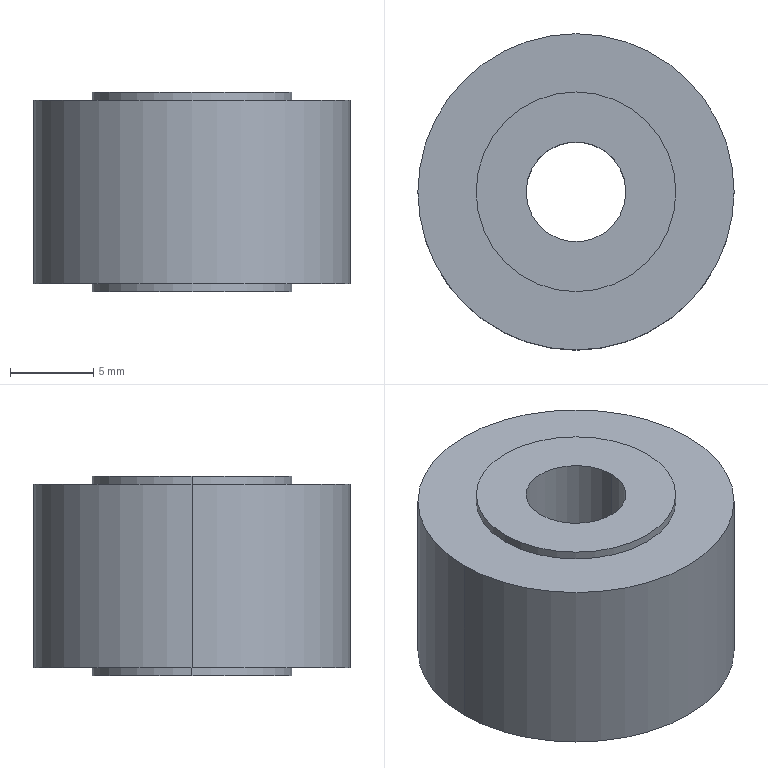Part | STEP file | 11-NARTR611 | 1 solid | 12 faces | box 19 x 19 x 12 mm | volume 2893 mm3 | cylinder 8 | plane 4 | commonest cylinder face diameters 12 x4 6 x2 19 x2
STEP:
#1=CARTESIAN_POINT('',(-6.,0.,-0.5));
#2=VERTEX_POINT('',#1);
#3=CARTESIAN_POINT('',(6.,0.,-0.5));
#4=VERTEX_POINT('',#3);
#5=CARTESIAN_POINT('',(0.,0.,-0.5));
#6=DIRECTION('',(0.,0.,-1.));
#7=DIRECTION('',(-1.,0.,0.));
#8=AXIS2_PLACEMENT_3D('',#5,#6,#7);
#9=CIRCLE('',#8,6.);
#10=EDGE_CURVE('',#2,#4,#9,.T.);
#11=ORIENTED_EDGE('',*,*,#10,.F.);
#12=CARTESIAN_POINT('',(-6.,0.,0.));
#13=VERTEX_POINT('',#12);
#14=CARTESIAN_POINT('',(-6.,0.,-0.5));
#15=DIRECTION('',(0.,0.,1.));
#16=VECTOR('',#15,1000.);
#17=LINE('',#14,#16);
#18=EDGE_CURVE('',#2,#13,#17,.T.);
#19=ORIENTED_EDGE('',*,*,#18,.T.);
#20=CARTESIAN_POINT('',(6.,0.,0.));
#21=VERTEX_POINT('',#20);
#22=CARTESIAN_POINT('',(0.,0.,0.));
#23=DIRECTION('',(0.,0.,-1.));
#24=DIRECTION('',(1.,0.,0.));
#25=AXIS2_PLACEMENT_3D('',#22,#23,#24);
#26=CIRCLE('',#25,6.);
#27=EDGE_CURVE('',#13,#21,#26,.T.);
#28=ORIENTED_EDGE('',*,*,#27,.T.);
#29=CARTESIAN_POINT('',(6.,0.,-0.5));
#30=DIRECTION('',(0.,0.,1.));
#31=VECTOR('',#30,1000.);
#32=LINE('',#29,#31);
#33=EDGE_CURVE('',#4,#21,#32,.T.);
#34=ORIENTED_EDGE('',*,*,#33,.F.);
#35=EDGE_LOOP('',(#11,#19,#28,#34));
#36=FACE_OUTER_BOUND('',#35,.T.);
#37=CARTESIAN_POINT('',(0.,0.,-0.5));
#38=DIRECTION('',(0.,0.,1.));
#39=DIRECTION('',(1.,0.,0.));
#40=AXIS2_PLACEMENT_3D('',#37,#38,#39);
#41=CYLINDRICAL_SURFACE('',#40,6.);
#42=ADVANCED_FACE('',(#36),#41,.T.);
#43=CARTESIAN_POINT('',(6.,0.,11.5));
#44=VERTEX_POINT('',#43);
#45=CARTESIAN_POINT('',(-6.,0.,11.5));
#46=VERTEX_POINT('',#45);
#47=CARTESIAN_POINT('',(0.,0.,11.5));
#48=DIRECTION('',(0.,0.,1.));
#49=DIRECTION('',(1.,0.,0.));
#50=AXIS2_PLACEMENT_3D('',#47,#48,#49);
#51=CIRCLE('',#50,6.);
#52=EDGE_CURVE('',#44,#46,#51,.T.);
#53=ORIENTED_EDGE('',*,*,#52,.F.);
#54=CARTESIAN_POINT('',(6.,0.,11.));
#55=VERTEX_POINT('',#54);
#56=CARTESIAN_POINT('',(6.,0.,11.5));
#57=DIRECTION('',(0.,0.,-1.));
#58=VECTOR('',#57,1000.);
#59=LINE('',#56,#58);
#60=EDGE_CURVE('',#44,#55,#59,.T.);
#61=ORIENTED_EDGE('',*,*,#60,.T.);
#62=CARTESIAN_POINT('',(-6.,0.,11.));
#63=VERTEX_POINT('',#62);
#64=CARTESIAN_POINT('',(0.,0.,11.));
#65=DIRECTION('',(0.,0.,1.));
#66=DIRECTION('',(1.,0.,0.));
#67=AXIS2_PLACEMENT_3D('',#64,#65,#66);
#68=CIRCLE('',#67,6.);
#69=EDGE_CURVE('',#55,#63,#68,.T.);
#70=ORIENTED_EDGE('',*,*,#69,.T.);
#71=CARTESIAN_POINT('',(-6.,0.,11.5));
#72=DIRECTION('',(0.,0.,-1.));
#73=VECTOR('',#72,1000.);
#74=LINE('',#71,#73);
#75=EDGE_CURVE('',#46,#63,#74,.T.);
#76=ORIENTED_EDGE('',*,*,#75,.F.);
#77=EDGE_LOOP('',(#53,#61,#70,#76));
#78=FACE_OUTER_BOUND('',#77,.T.);
#79=CARTESIAN_POINT('',(0.,0.,11.5));
#80=DIRECTION('',(0.,0.,-1.));
#81=DIRECTION('',(-1.,0.,0.));
#82=AXIS2_PLACEMENT_3D('',#79,#80,#81);
#83=CYLINDRICAL_SURFACE('',#82,6.);
#84=ADVANCED_FACE('',(#78),#83,.T.);
#85=CARTESIAN_POINT('',(-3.,0.,11.5));
#86=VERTEX_POINT('',#85);
#87=CARTESIAN_POINT('',(3.,0.,11.5));
#88=VERTEX_POINT('',#87);
#89=CARTESIAN_POINT('',(0.,0.,11.5));
#90=DIRECTION('',(0.,0.,1.));
#91=DIRECTION('',(1.,0.,0.));
#92=AXIS2_PLACEMENT_3D('',#89,#90,#91);
#93=CIRCLE('',#92,3.);
#94=EDGE_CURVE('',#86,#88,#93,.T.);
#95=ORIENTED_EDGE('',*,*,#94,.T.);
#96=CARTESIAN_POINT('',(3.,0.,-0.5));
#97=VERTEX_POINT('',#96);
#98=CARTESIAN_POINT('',(3.,0.,11.));
#99=DIRECTION('',(0.,0.,-1.));
#100=VECTOR('',#99,1000.);
#101=LINE('',#98,#100);
#102=EDGE_CURVE('',#88,#97,#101,.T.);
#103=ORIENTED_EDGE('',*,*,#102,.T.);
#104=CARTESIAN_POINT('',(-3.,0.,-0.5));
#105=VERTEX_POINT('',#104);
#106=CARTESIAN_POINT('',(0.,0.,-0.5));
#107=DIRECTION('',(0.,0.,-1.));
#108=DIRECTION('',(-1.,0.,0.));
#109=AXIS2_PLACEMENT_3D('',#106,#107,#108);
#110=CIRCLE('',#109,3.);
#111=EDGE_CURVE('',#97,#105,#110,.T.);
#112=ORIENTED_EDGE('',*,*,#111,.T.);
#113=CARTESIAN_POINT('',(-3.,0.,11.));
#114=DIRECTION('',(0.,0.,-1.));
#115=VECTOR('',#114,1000.);
#116=LINE('',#113,#115);
#117=EDGE_CURVE('',#86,#105,#116,.T.);
#118=ORIENTED_EDGE('',*,*,#117,.F.);
#119=EDGE_LOOP('',(#95,#103,#112,#118));
#120=FACE_OUTER_BOUND('',#119,.T.);
#121=CARTESIAN_POINT('',(0.,0.,11.));
#122=DIRECTION('',(0.,0.,-1.));
#123=DIRECTION('',(-1.,0.,0.));
#124=AXIS2_PLACEMENT_3D('',#121,#122,#123);
#125=CYLINDRICAL_SURFACE('',#124,3.);
#126=ADVANCED_FACE('',(#120),#125,.F.);
#127=CARTESIAN_POINT('',(9.5,0.,11.));
#128=VERTEX_POINT('',#127);
#129=CARTESIAN_POINT('',(-9.5,0.,11.));
#130=VERTEX_POINT('',#129);
#131=CARTESIAN_POINT('',(0.,0.,11.));
#132=DIRECTION('',(0.,0.,1.));
#133=DIRECTION('',(1.,0.,0.));
#134=AXIS2_PLACEMENT_3D('',#131,#132,#133);
#135=CIRCLE('',#134,9.5);
#136=EDGE_CURVE('',#128,#130,#135,.T.);
#137=ORIENTED_EDGE('',*,*,#136,.F.);
#138=CARTESIAN_POINT('',(9.5,0.,0.));
#139=VERTEX_POINT('',#138);
#140=CARTESIAN_POINT('',(9.5,0.,11.));
#141=DIRECTION('',(0.,0.,-1.));
#142=VECTOR('',#141,1000.);
#143=LINE('',#140,#142);
#144=EDGE_CURVE('',#128,#139,#143,.T.);
#145=ORIENTED_EDGE('',*,*,#144,.T.);
#146=CARTESIAN_POINT('',(-9.5,0.,0.));
#147=VERTEX_POINT('',#146);
#148=CARTESIAN_POINT('',(0.,0.,0.));
#149=DIRECTION('',(0.,0.,1.));
#150=DIRECTION('',(1.,0.,0.));
#151=AXIS2_PLACEMENT_3D('',#148,#149,#150);
#152=CIRCLE('',#151,9.5);
#153=EDGE_CURVE('',#139,#147,#152,.T.);
#154=ORIENTED_EDGE('',*,*,#153,.T.);
#155=CARTESIAN_POINT('',(-9.5,0.,11.));
#156=DIRECTION('',(0.,0.,-1.));
#157=VECTOR('',#156,1000.);
#158=LINE('',#155,#157);
#159=EDGE_CURVE('',#130,#147,#158,.T.);
#160=ORIENTED_EDGE('',*,*,#159,.F.);
#161=EDGE_LOOP('',(#137,#145,#154,#160));
#162=FACE_OUTER_BOUND('',#161,.T.);
#163=CARTESIAN_POINT('',(0.,0.,11.));
#164=DIRECTION('',(0.,0.,-1.));
#165=DIRECTION('',(-1.,0.,0.));
#166=AXIS2_PLACEMENT_3D('',#163,#164,#165);
#167=CYLINDRICAL_SURFACE('',#166,9.5);
#168=ADVANCED_FACE('',(#162),#167,.T.);
#169=CARTESIAN_POINT('',(0.,0.,0.));
#170=DIRECTION('',(0.,0.,1.));
#171=DIRECTION('',(1.,0.,0.));
#172=AXIS2_PLACEMENT_3D('',#169,#170,#171);
#173=CIRCLE('',#172,9.5);
#174=EDGE_CURVE('',#147,#139,#173,.T.);
#175=ORIENTED_EDGE('',*,*,#174,.F.);
#176=ORIENTED_EDGE('',*,*,#153,.F.);
#177=EDGE_LOOP('',(#175,#176));
#178=FACE_OUTER_BOUND('',#177,.T.);
#179=CARTESIAN_POINT('',(0.,0.,0.));
#180=DIRECTION('',(0.,0.,-1.));
#181=DIRECTION('',(1.,0.,0.));
#182=AXIS2_PLACEMENT_3D('',#179,#180,#181);
#183=CIRCLE('',#182,6.);
#184=EDGE_CURVE('',#21,#13,#183,.T.);
#185=ORIENTED_EDGE('',*,*,#184,.F.);
#186=ORIENTED_EDGE('',*,*,#27,.F.);
#187=EDGE_LOOP('',(#185,#186));
#188=FACE_BOUND('',#187,.T.);
#189=CARTESIAN_POINT('',(0.,0.,0.));
#190=DIRECTION('',(0.,0.,1.));
#191=DIRECTION('',(1.,0.,0.));
#192=AXIS2_PLACEMENT_3D('',#189,#190,#191);
#193=PLANE('',#192);
#194=ADVANCED_FACE('',(#178,#188),#193,.F.);
#195=CARTESIAN_POINT('',(0.,0.,11.));
#196=DIRECTION('',(0.,0.,1.));
#197=DIRECTION('',(1.,0.,0.));
#198=AXIS2_PLACEMENT_3D('',#195,#196,#197);
#199=CIRCLE('',#198,9.5);
#200=EDGE_CURVE('',#130,#128,#199,.T.);
#201=ORIENTED_EDGE('',*,*,#200,.T.);
#202=ORIENTED_EDGE('',*,*,#136,.T.);
#203=EDGE_LOOP('',(#201,#202));
#204=FACE_OUTER_BOUND('',#203,.T.);
#205=CARTESIAN_POINT('',(0.,0.,11.));
#206=DIRECTION('',(0.,0.,1.));
#207=DIRECTION('',(1.,0.,0.));
#208=AXIS2_PLACEMENT_3D('',#205,#206,#207);
#209=CIRCLE('',#208,6.);
#210=EDGE_CURVE('',#63,#55,#209,.T.);
#211=ORIENTED_EDGE('',*,*,#210,.F.);
#212=ORIENTED_EDGE('',*,*,#69,.F.);
#213=EDGE_LOOP('',(#211,#212));
#214=FACE_BOUND('',#213,.T.);
#215=CARTESIAN_POINT('',(0.,0.,11.));
#216=DIRECTION('',(0.,0.,1.));
#217=DIRECTION('',(1.,0.,0.));
#218=AXIS2_PLACEMENT_3D('',#215,#216,#217);
#219=PLANE('',#218);
#220=ADVANCED_FACE('',(#204,#214),#219,.T.);
#221=ORIENTED_EDGE('',*,*,#144,.F.);
#222=ORIENTED_EDGE('',*,*,#200,.F.);
#223=ORIENTED_EDGE('',*,*,#159,.T.);
#224=ORIENTED_EDGE('',*,*,#174,.T.);
#225=EDGE_LOOP('',(#221,#222,#223,#224));
#226=FACE_OUTER_BOUND('',#225,.T.);
#227=CARTESIAN_POINT('',(0.,0.,11.));
#228=DIRECTION('',(0.,0.,-1.));
#229=DIRECTION('',(-1.,0.,0.));
#230=AXIS2_PLACEMENT_3D('',#227,#228,#229);
#231=CYLINDRICAL_SURFACE('',#230,9.5);
#232=ADVANCED_FACE('',(#226),#231,.T.);
#233=ORIENTED_EDGE('',*,*,#102,.F.);
#234=CARTESIAN_POINT('',(0.,0.,11.5));
#235=DIRECTION('',(0.,0.,1.));
#236=DIRECTION('',(1.,0.,0.));
#237=AXIS2_PLACEMENT_3D('',#234,#235,#236);
#238=CIRCLE('',#237,3.);
#239=EDGE_CURVE('',#88,#86,#238,.T.);
#240=ORIENTED_EDGE('',*,*,#239,.T.);
#241=ORIENTED_EDGE('',*,*,#117,.T.);
#242=CARTESIAN_POINT('',(0.,0.,-0.5));
#243=DIRECTION('',(0.,0.,-1.));
#244=DIRECTION('',(-1.,0.,0.));
#245=AXIS2_PLACEMENT_3D('',#242,#243,#244);
#246=CIRCLE('',#245,3.);
#247=EDGE_CURVE('',#105,#97,#246,.T.);
#248=ORIENTED_EDGE('',*,*,#247,.T.);
#249=EDGE_LOOP('',(#233,#240,#241,#248));
#250=FACE_OUTER_BOUND('',#249,.T.);
#251=CARTESIAN_POINT('',(0.,0.,11.));
#252=DIRECTION('',(0.,0.,-1.));
#253=DIRECTION('',(-1.,0.,0.));
#254=AXIS2_PLACEMENT_3D('',#251,#252,#253);
#255=CYLINDRICAL_SURFACE('',#254,3.);
#256=ADVANCED_FACE('',(#250),#255,.F.);
#257=CARTESIAN_POINT('',(0.,0.,11.5));
#258=DIRECTION('',(0.,0.,1.));
#259=DIRECTION('',(1.,0.,0.));
#260=AXIS2_PLACEMENT_3D('',#257,#258,#259);
#261=CIRCLE('',#260,6.);
#262=EDGE_CURVE('',#46,#44,#261,.T.);
#263=ORIENTED_EDGE('',*,*,#262,.T.);
#264=ORIENTED_EDGE('',*,*,#52,.T.);
#265=EDGE_LOOP('',(#263,#264));
#266=FACE_OUTER_BOUND('',#265,.T.);
#267=ORIENTED_EDGE('',*,*,#94,.F.);
#268=ORIENTED_EDGE('',*,*,#239,.F.);
#269=EDGE_LOOP('',(#267,#268));
#270=FACE_BOUND('',#269,.T.);
#271=CARTESIAN_POINT('',(0.,0.,11.5));
#272=DIRECTION('',(0.,0.,1.));
#273=DIRECTION('',(1.,0.,0.));
#274=AXIS2_PLACEMENT_3D('',#271,#272,#273);
#275=PLANE('',#274);
#276=ADVANCED_FACE('',(#266,#270),#275,.T.);
#277=ORIENTED_EDGE('',*,*,#60,.F.);
#278=ORIENTED_EDGE('',*,*,#262,.F.);
#279=ORIENTED_EDGE('',*,*,#75,.T.);
#280=ORIENTED_EDGE('',*,*,#210,.T.);
#281=EDGE_LOOP('',(#277,#278,#279,#280));
#282=FACE_OUTER_BOUND('',#281,.T.);
#283=CARTESIAN_POINT('',(0.,0.,11.5));
#284=DIRECTION('',(0.,0.,-1.));
#285=DIRECTION('',(-1.,0.,0.));
#286=AXIS2_PLACEMENT_3D('',#283,#284,#285);
#287=CYLINDRICAL_SURFACE('',#286,6.);
#288=ADVANCED_FACE('',(#282),#287,.T.);
#289=CARTESIAN_POINT('',(0.,0.,-0.5));
#290=DIRECTION('',(0.,0.,-1.));
#291=DIRECTION('',(-1.,0.,0.));
#292=AXIS2_PLACEMENT_3D('',#289,#290,#291);
#293=CIRCLE('',#292,6.);
#294=EDGE_CURVE('',#4,#2,#293,.T.);
#295=ORIENTED_EDGE('',*,*,#294,.T.);
#296=ORIENTED_EDGE('',*,*,#10,.T.);
#297=EDGE_LOOP('',(#295,#296));
#298=FACE_OUTER_BOUND('',#297,.T.);
#299=ORIENTED_EDGE('',*,*,#247,.F.);
#300=ORIENTED_EDGE('',*,*,#111,.F.);
#301=EDGE_LOOP('',(#299,#300));
#302=FACE_BOUND('',#301,.T.);
#303=CARTESIAN_POINT('',(0.,0.,-0.5));
#304=DIRECTION('',(0.,0.,-1.));
#305=DIRECTION('',(-1.,0.,0.));
#306=AXIS2_PLACEMENT_3D('',#303,#304,#305);
#307=PLANE('',#306);
#308=ADVANCED_FACE('',(#298,#302),#307,.T.);
#309=ORIENTED_EDGE('',*,*,#18,.F.);
#310=ORIENTED_EDGE('',*,*,#294,.F.);
#311=ORIENTED_EDGE('',*,*,#33,.T.);
#312=ORIENTED_EDGE('',*,*,#184,.T.);
#313=EDGE_LOOP('',(#309,#310,#311,#312));
#314=FACE_OUTER_BOUND('',#313,.T.);
#315=CARTESIAN_POINT('',(0.,0.,-0.5));
#316=DIRECTION('',(0.,0.,1.));
#317=DIRECTION('',(1.,0.,0.));
#318=AXIS2_PLACEMENT_3D('',#315,#316,#317);
#319=CYLINDRICAL_SURFACE('',#318,6.);
#320=ADVANCED_FACE('',(#314),#319,.T.);
#321=CLOSED_SHELL('',(#42,#84,#126,#168,#194,#220,#232,#256,#276,#288,#308,#320));
#322=MANIFOLD_SOLID_BREP('',#321);
#323=CARTESIAN_POINT('',(0.,0.,0.));
#324=DIRECTION('',(0.,0.,1.));
#325=DIRECTION('',(1.,0.,0.));
#326=AXIS2_PLACEMENT_3D('',#323,#324,#325);
#327=(LENGTH_UNIT()NAMED_UNIT(*)SI_UNIT(.MILLI.,.METRE.));
#328=UNCERTAINTY_MEASURE_WITH_UNIT(LENGTH_MEASURE(0.00001),#327,'','');
#329=(NAMED_UNIT(*)PLANE_ANGLE_UNIT()SI_UNIT($,.RADIAN.));
#330=(NAMED_UNIT(*)SI_UNIT($,.STERADIAN.)SOLID_ANGLE_UNIT());
#331=(GEOMETRIC_REPRESENTATION_CONTEXT(3)GLOBAL_UNCERTAINTY_ASSIGNED_CONTEXT((#328))GLOBAL_UNIT_ASSIGNED_CONTEXT((#327,#329,#330))REPRESENTATION_CONTEXT('',''));
#332=ADVANCED_BREP_SHAPE_REPRESENTATION('',(#322,#326),#331);